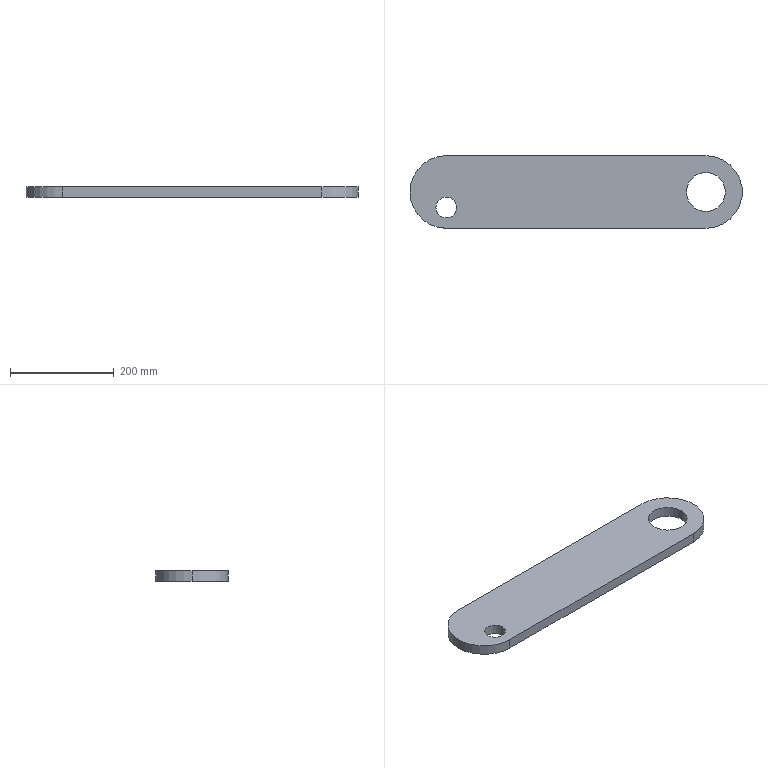Part | SolidWorks | features Extrusion 1 | 1 solid | 11 faces | box 640 x 140 x 20 mm | volume 1594386 mm3 | cylinder 7 | plane 4 | commonest cylinder face diameters 140 x3 40 x2 75 x2
STEP:
#1=CARTESIAN_POINT('',(-270.,-30.,20.));
#2=VERTEX_POINT('',#1);
#3=CARTESIAN_POINT('',(-230.,-30.,20.));
#4=VERTEX_POINT('',#3);
#5=CARTESIAN_POINT('',(-250.,-30.,20.));
#6=DIRECTION('',(0.,0.,1.));
#7=DIRECTION('',(1.,0.,0.));
#8=AXIS2_PLACEMENT_3D('',#5,#6,#7);
#9=CIRCLE('',#8,20.);
#10=EDGE_CURVE('',#2,#4,#9,.T.);
#11=ORIENTED_EDGE('',*,*,#10,.T.);
#12=CARTESIAN_POINT('',(-230.,-30.,0.));
#13=VERTEX_POINT('',#12);
#14=CARTESIAN_POINT('',(-230.,-30.,20.));
#15=DIRECTION('',(0.,0.,-1.));
#16=VECTOR('',#15,1000.);
#17=LINE('',#14,#16);
#18=EDGE_CURVE('',#4,#13,#17,.T.);
#19=ORIENTED_EDGE('',*,*,#18,.T.);
#20=CARTESIAN_POINT('',(-270.,-30.,0.));
#21=VERTEX_POINT('',#20);
#22=CARTESIAN_POINT('',(-250.,-30.,0.));
#23=DIRECTION('',(0.,0.,1.));
#24=DIRECTION('',(1.,0.,0.));
#25=AXIS2_PLACEMENT_3D('',#22,#23,#24);
#26=CIRCLE('',#25,20.);
#27=EDGE_CURVE('',#21,#13,#26,.T.);
#28=ORIENTED_EDGE('',*,*,#27,.F.);
#29=CARTESIAN_POINT('',(-270.,-30.,20.));
#30=DIRECTION('',(0.,0.,-1.));
#31=VECTOR('',#30,1000.);
#32=LINE('',#29,#31);
#33=EDGE_CURVE('',#2,#21,#32,.T.);
#34=ORIENTED_EDGE('',*,*,#33,.F.);
#35=EDGE_LOOP('',(#11,#19,#28,#34));
#36=FACE_OUTER_BOUND('',#35,.T.);
#37=CARTESIAN_POINT('',(-250.,-30.,20.));
#38=DIRECTION('',(0.,0.,-1.));
#39=DIRECTION('',(-1.,0.,0.));
#40=AXIS2_PLACEMENT_3D('',#37,#38,#39);
#41=CYLINDRICAL_SURFACE('',#40,20.);
#42=ADVANCED_FACE('',(#36),#41,.F.);
#43=CARTESIAN_POINT('',(212.5,0.,20.));
#44=VERTEX_POINT('',#43);
#45=CARTESIAN_POINT('',(287.5,0.,20.));
#46=VERTEX_POINT('',#45);
#47=CARTESIAN_POINT('',(250.,0.,20.));
#48=DIRECTION('',(0.,0.,1.));
#49=DIRECTION('',(1.,0.,0.));
#50=AXIS2_PLACEMENT_3D('',#47,#48,#49);
#51=CIRCLE('',#50,37.5);
#52=EDGE_CURVE('',#44,#46,#51,.T.);
#53=ORIENTED_EDGE('',*,*,#52,.T.);
#54=CARTESIAN_POINT('',(287.5,0.,0.));
#55=VERTEX_POINT('',#54);
#56=CARTESIAN_POINT('',(287.5,0.,20.));
#57=DIRECTION('',(0.,0.,-1.));
#58=VECTOR('',#57,1000.);
#59=LINE('',#56,#58);
#60=EDGE_CURVE('',#46,#55,#59,.T.);
#61=ORIENTED_EDGE('',*,*,#60,.T.);
#62=CARTESIAN_POINT('',(212.5,0.,0.));
#63=VERTEX_POINT('',#62);
#64=CARTESIAN_POINT('',(250.,0.,0.));
#65=DIRECTION('',(0.,0.,1.));
#66=DIRECTION('',(1.,0.,0.));
#67=AXIS2_PLACEMENT_3D('',#64,#65,#66);
#68=CIRCLE('',#67,37.5);
#69=EDGE_CURVE('',#63,#55,#68,.T.);
#70=ORIENTED_EDGE('',*,*,#69,.F.);
#71=CARTESIAN_POINT('',(212.5,0.,20.));
#72=DIRECTION('',(0.,0.,-1.));
#73=VECTOR('',#72,1000.);
#74=LINE('',#71,#73);
#75=EDGE_CURVE('',#44,#63,#74,.T.);
#76=ORIENTED_EDGE('',*,*,#75,.F.);
#77=EDGE_LOOP('',(#53,#61,#70,#76));
#78=FACE_OUTER_BOUND('',#77,.T.);
#79=CARTESIAN_POINT('',(250.,0.,20.));
#80=DIRECTION('',(0.,0.,-1.));
#81=DIRECTION('',(-1.,0.,0.));
#82=AXIS2_PLACEMENT_3D('',#79,#80,#81);
#83=CYLINDRICAL_SURFACE('',#82,37.5);
#84=ADVANCED_FACE('',(#78),#83,.F.);
#85=CARTESIAN_POINT('',(-320.,0.,20.));
#86=VERTEX_POINT('',#85);
#87=CARTESIAN_POINT('',(-250.,-70.,20.));
#88=VERTEX_POINT('',#87);
#89=CARTESIAN_POINT('',(-250.,0.,20.));
#90=DIRECTION('',(0.,0.,1.));
#91=DIRECTION('',(1.,0.,0.));
#92=AXIS2_PLACEMENT_3D('',#89,#90,#91);
#93=CIRCLE('',#92,70.);
#94=EDGE_CURVE('',#86,#88,#93,.T.);
#95=ORIENTED_EDGE('',*,*,#94,.F.);
#96=CARTESIAN_POINT('',(-320.,0.,0.));
#97=VERTEX_POINT('',#96);
#98=CARTESIAN_POINT('',(-320.,0.,20.));
#99=DIRECTION('',(0.,0.,-1.));
#100=VECTOR('',#99,1000.);
#101=LINE('',#98,#100);
#102=EDGE_CURVE('',#86,#97,#101,.T.);
#103=ORIENTED_EDGE('',*,*,#102,.T.);
#104=CARTESIAN_POINT('',(-250.,-70.,0.));
#105=VERTEX_POINT('',#104);
#106=CARTESIAN_POINT('',(-250.,0.,0.));
#107=DIRECTION('',(0.,0.,1.));
#108=DIRECTION('',(1.,0.,0.));
#109=AXIS2_PLACEMENT_3D('',#106,#107,#108);
#110=CIRCLE('',#109,70.);
#111=EDGE_CURVE('',#97,#105,#110,.T.);
#112=ORIENTED_EDGE('',*,*,#111,.T.);
#113=CARTESIAN_POINT('',(-250.,-70.,20.));
#114=DIRECTION('',(0.,0.,-1.));
#115=VECTOR('',#114,1000.);
#116=LINE('',#113,#115);
#117=EDGE_CURVE('',#88,#105,#116,.T.);
#118=ORIENTED_EDGE('',*,*,#117,.F.);
#119=EDGE_LOOP('',(#95,#103,#112,#118));
#120=FACE_OUTER_BOUND('',#119,.T.);
#121=CARTESIAN_POINT('',(-250.,0.,20.));
#122=DIRECTION('',(0.,0.,-1.));
#123=DIRECTION('',(-1.,0.,0.));
#124=AXIS2_PLACEMENT_3D('',#121,#122,#123);
#125=CYLINDRICAL_SURFACE('',#124,70.);
#126=ADVANCED_FACE('',(#120),#125,.T.);
#127=ORIENTED_EDGE('',*,*,#52,.F.);
#128=CARTESIAN_POINT('',(250.,0.,20.));
#129=DIRECTION('',(0.,0.,1.));
#130=DIRECTION('',(1.,0.,0.));
#131=AXIS2_PLACEMENT_3D('',#128,#129,#130);
#132=CIRCLE('',#131,37.5);
#133=EDGE_CURVE('',#46,#44,#132,.T.);
#134=ORIENTED_EDGE('',*,*,#133,.F.);
#135=EDGE_LOOP('',(#127,#134));
#136=FACE_BOUND('',#135,.T.);
#137=CARTESIAN_POINT('',(-250.,70.,20.));
#138=VERTEX_POINT('',#137);
#139=CARTESIAN_POINT('',(-250.,0.,20.));
#140=DIRECTION('',(0.,0.,1.));
#141=DIRECTION('',(1.,0.,0.));
#142=AXIS2_PLACEMENT_3D('',#139,#140,#141);
#143=CIRCLE('',#142,70.);
#144=EDGE_CURVE('',#138,#86,#143,.T.);
#145=ORIENTED_EDGE('',*,*,#144,.T.);
#146=ORIENTED_EDGE('',*,*,#94,.T.);
#147=CARTESIAN_POINT('',(250.,-70.,20.));
#148=VERTEX_POINT('',#147);
#149=CARTESIAN_POINT('',(-250.,-70.,20.));
#150=DIRECTION('',(1.,0.,0.));
#151=VECTOR('',#150,1000.);
#152=LINE('',#149,#151);
#153=EDGE_CURVE('',#88,#148,#152,.T.);
#154=ORIENTED_EDGE('',*,*,#153,.T.);
#155=CARTESIAN_POINT('',(250.,70.,20.));
#156=VERTEX_POINT('',#155);
#157=CARTESIAN_POINT('',(250.,0.,20.));
#158=DIRECTION('',(0.,0.,1.));
#159=DIRECTION('',(1.,0.,0.));
#160=AXIS2_PLACEMENT_3D('',#157,#158,#159);
#161=CIRCLE('',#160,70.);
#162=EDGE_CURVE('',#148,#156,#161,.T.);
#163=ORIENTED_EDGE('',*,*,#162,.T.);
#164=CARTESIAN_POINT('',(-250.,70.,20.));
#165=DIRECTION('',(-1.,0.,0.));
#166=VECTOR('',#165,1000.);
#167=LINE('',#164,#166);
#168=EDGE_CURVE('',#156,#138,#167,.T.);
#169=ORIENTED_EDGE('',*,*,#168,.T.);
#170=EDGE_LOOP('',(#145,#146,#154,#163,#169));
#171=FACE_OUTER_BOUND('',#170,.T.);
#172=ORIENTED_EDGE('',*,*,#10,.F.);
#173=CARTESIAN_POINT('',(-250.,-30.,20.));
#174=DIRECTION('',(0.,0.,1.));
#175=DIRECTION('',(1.,0.,0.));
#176=AXIS2_PLACEMENT_3D('',#173,#174,#175);
#177=CIRCLE('',#176,20.);
#178=EDGE_CURVE('',#4,#2,#177,.T.);
#179=ORIENTED_EDGE('',*,*,#178,.F.);
#180=EDGE_LOOP('',(#172,#179));
#181=FACE_BOUND('',#180,.T.);
#182=CARTESIAN_POINT('',(-250.,0.,20.));
#183=DIRECTION('',(0.,0.,1.));
#184=DIRECTION('',(1.,0.,0.));
#185=AXIS2_PLACEMENT_3D('',#182,#183,#184);
#186=PLANE('',#185);
#187=ADVANCED_FACE('',(#136,#171,#181),#186,.T.);
#188=CARTESIAN_POINT('',(-250.,70.,0.));
#189=VERTEX_POINT('',#188);
#190=CARTESIAN_POINT('',(-250.,0.,0.));
#191=DIRECTION('',(0.,0.,1.));
#192=DIRECTION('',(1.,0.,0.));
#193=AXIS2_PLACEMENT_3D('',#190,#191,#192);
#194=CIRCLE('',#193,70.);
#195=EDGE_CURVE('',#189,#97,#194,.T.);
#196=ORIENTED_EDGE('',*,*,#195,.F.);
#197=CARTESIAN_POINT('',(250.,70.,0.));
#198=VERTEX_POINT('',#197);
#199=CARTESIAN_POINT('',(-250.,70.,0.));
#200=DIRECTION('',(-1.,0.,0.));
#201=VECTOR('',#200,1000.);
#202=LINE('',#199,#201);
#203=EDGE_CURVE('',#198,#189,#202,.T.);
#204=ORIENTED_EDGE('',*,*,#203,.F.);
#205=CARTESIAN_POINT('',(250.,-70.,0.));
#206=VERTEX_POINT('',#205);
#207=CARTESIAN_POINT('',(250.,0.,0.));
#208=DIRECTION('',(0.,0.,1.));
#209=DIRECTION('',(1.,0.,0.));
#210=AXIS2_PLACEMENT_3D('',#207,#208,#209);
#211=CIRCLE('',#210,70.);
#212=EDGE_CURVE('',#206,#198,#211,.T.);
#213=ORIENTED_EDGE('',*,*,#212,.F.);
#214=CARTESIAN_POINT('',(-250.,-70.,0.));
#215=DIRECTION('',(1.,0.,0.));
#216=VECTOR('',#215,1000.);
#217=LINE('',#214,#216);
#218=EDGE_CURVE('',#105,#206,#217,.T.);
#219=ORIENTED_EDGE('',*,*,#218,.F.);
#220=ORIENTED_EDGE('',*,*,#111,.F.);
#221=EDGE_LOOP('',(#196,#204,#213,#219,#220));
#222=FACE_OUTER_BOUND('',#221,.T.);
#223=ORIENTED_EDGE('',*,*,#69,.T.);
#224=CARTESIAN_POINT('',(250.,0.,0.));
#225=DIRECTION('',(0.,0.,1.));
#226=DIRECTION('',(1.,0.,0.));
#227=AXIS2_PLACEMENT_3D('',#224,#225,#226);
#228=CIRCLE('',#227,37.5);
#229=EDGE_CURVE('',#55,#63,#228,.T.);
#230=ORIENTED_EDGE('',*,*,#229,.T.);
#231=EDGE_LOOP('',(#223,#230));
#232=FACE_BOUND('',#231,.T.);
#233=ORIENTED_EDGE('',*,*,#27,.T.);
#234=CARTESIAN_POINT('',(-250.,-30.,0.));
#235=DIRECTION('',(0.,0.,1.));
#236=DIRECTION('',(1.,0.,0.));
#237=AXIS2_PLACEMENT_3D('',#234,#235,#236);
#238=CIRCLE('',#237,20.);
#239=EDGE_CURVE('',#13,#21,#238,.T.);
#240=ORIENTED_EDGE('',*,*,#239,.T.);
#241=EDGE_LOOP('',(#233,#240));
#242=FACE_BOUND('',#241,.T.);
#243=CARTESIAN_POINT('',(-250.,0.,0.));
#244=DIRECTION('',(0.,0.,1.));
#245=DIRECTION('',(1.,0.,0.));
#246=AXIS2_PLACEMENT_3D('',#243,#244,#245);
#247=PLANE('',#246);
#248=ADVANCED_FACE('',(#222,#232,#242),#247,.F.);
#249=ORIENTED_EDGE('',*,*,#102,.F.);
#250=ORIENTED_EDGE('',*,*,#144,.F.);
#251=CARTESIAN_POINT('',(-250.,70.,20.));
#252=DIRECTION('',(0.,0.,-1.));
#253=VECTOR('',#252,1000.);
#254=LINE('',#251,#253);
#255=EDGE_CURVE('',#138,#189,#254,.T.);
#256=ORIENTED_EDGE('',*,*,#255,.T.);
#257=ORIENTED_EDGE('',*,*,#195,.T.);
#258=EDGE_LOOP('',(#249,#250,#256,#257));
#259=FACE_OUTER_BOUND('',#258,.T.);
#260=CARTESIAN_POINT('',(-250.,0.,20.));
#261=DIRECTION('',(0.,0.,-1.));
#262=DIRECTION('',(-1.,0.,0.));
#263=AXIS2_PLACEMENT_3D('',#260,#261,#262);
#264=CYLINDRICAL_SURFACE('',#263,70.);
#265=ADVANCED_FACE('',(#259),#264,.T.);
#266=ORIENTED_EDGE('',*,*,#218,.T.);
#267=CARTESIAN_POINT('',(250.,-70.,20.));
#268=DIRECTION('',(0.,0.,-1.));
#269=VECTOR('',#268,1000.);
#270=LINE('',#267,#269);
#271=EDGE_CURVE('',#148,#206,#270,.T.);
#272=ORIENTED_EDGE('',*,*,#271,.F.);
#273=ORIENTED_EDGE('',*,*,#153,.F.);
#274=ORIENTED_EDGE('',*,*,#117,.T.);
#275=EDGE_LOOP('',(#266,#272,#273,#274));
#276=FACE_OUTER_BOUND('',#275,.T.);
#277=CARTESIAN_POINT('',(-250.,-70.,20.));
#278=DIRECTION('',(0.,1.,0.));
#279=DIRECTION('',(-1.,0.,0.));
#280=AXIS2_PLACEMENT_3D('',#277,#278,#279);
#281=PLANE('',#280);
#282=ADVANCED_FACE('',(#276),#281,.F.);
#283=ORIENTED_EDGE('',*,*,#212,.T.);
#284=CARTESIAN_POINT('',(250.,70.,20.));
#285=DIRECTION('',(0.,0.,-1.));
#286=VECTOR('',#285,1000.);
#287=LINE('',#284,#286);
#288=EDGE_CURVE('',#156,#198,#287,.T.);
#289=ORIENTED_EDGE('',*,*,#288,.F.);
#290=ORIENTED_EDGE('',*,*,#162,.F.);
#291=ORIENTED_EDGE('',*,*,#271,.T.);
#292=EDGE_LOOP('',(#283,#289,#290,#291));
#293=FACE_OUTER_BOUND('',#292,.T.);
#294=CARTESIAN_POINT('',(250.,0.,20.));
#295=DIRECTION('',(0.,0.,-1.));
#296=DIRECTION('',(-1.,0.,0.));
#297=AXIS2_PLACEMENT_3D('',#294,#295,#296);
#298=CYLINDRICAL_SURFACE('',#297,70.);
#299=ADVANCED_FACE('',(#293),#298,.T.);
#300=ORIENTED_EDGE('',*,*,#203,.T.);
#301=ORIENTED_EDGE('',*,*,#255,.F.);
#302=ORIENTED_EDGE('',*,*,#168,.F.);
#303=ORIENTED_EDGE('',*,*,#288,.T.);
#304=EDGE_LOOP('',(#300,#301,#302,#303));
#305=FACE_OUTER_BOUND('',#304,.T.);
#306=CARTESIAN_POINT('',(-250.,70.,20.));
#307=DIRECTION('',(0.,-1.,0.));
#308=DIRECTION('',(1.,0.,0.));
#309=AXIS2_PLACEMENT_3D('',#306,#307,#308);
#310=PLANE('',#309);
#311=ADVANCED_FACE('',(#305),#310,.F.);
#312=ORIENTED_EDGE('',*,*,#60,.F.);
#313=ORIENTED_EDGE('',*,*,#133,.T.);
#314=ORIENTED_EDGE('',*,*,#75,.T.);
#315=ORIENTED_EDGE('',*,*,#229,.F.);
#316=EDGE_LOOP('',(#312,#313,#314,#315));
#317=FACE_OUTER_BOUND('',#316,.T.);
#318=CARTESIAN_POINT('',(250.,0.,20.));
#319=DIRECTION('',(0.,0.,-1.));
#320=DIRECTION('',(-1.,0.,0.));
#321=AXIS2_PLACEMENT_3D('',#318,#319,#320);
#322=CYLINDRICAL_SURFACE('',#321,37.5);
#323=ADVANCED_FACE('',(#317),#322,.F.);
#324=ORIENTED_EDGE('',*,*,#18,.F.);
#325=ORIENTED_EDGE('',*,*,#178,.T.);
#326=ORIENTED_EDGE('',*,*,#33,.T.);
#327=ORIENTED_EDGE('',*,*,#239,.F.);
#328=EDGE_LOOP('',(#324,#325,#326,#327));
#329=FACE_OUTER_BOUND('',#328,.T.);
#330=CARTESIAN_POINT('',(-250.,-30.,20.));
#331=DIRECTION('',(0.,0.,-1.));
#332=DIRECTION('',(-1.,0.,0.));
#333=AXIS2_PLACEMENT_3D('',#330,#331,#332);
#334=CYLINDRICAL_SURFACE('',#333,20.);
#335=ADVANCED_FACE('',(#329),#334,.F.);
#336=CLOSED_SHELL('',(#42,#84,#126,#187,#248,#265,#282,#299,#311,#323,#335));
#337=MANIFOLD_SOLID_BREP('',#336);
#338=CARTESIAN_POINT('',(0.,0.,0.));
#339=DIRECTION('',(0.,0.,1.));
#340=DIRECTION('',(1.,0.,0.));
#341=AXIS2_PLACEMENT_3D('',#338,#339,#340);
#342=(LENGTH_UNIT()NAMED_UNIT(*)SI_UNIT(.MILLI.,.METRE.));
#343=UNCERTAINTY_MEASURE_WITH_UNIT(LENGTH_MEASURE(0.00001),#342,'','');
#344=(NAMED_UNIT(*)PLANE_ANGLE_UNIT()SI_UNIT($,.RADIAN.));
#345=(NAMED_UNIT(*)SI_UNIT($,.STERADIAN.)SOLID_ANGLE_UNIT());
#346=(GEOMETRIC_REPRESENTATION_CONTEXT(3)GLOBAL_UNCERTAINTY_ASSIGNED_CONTEXT((#343))GLOBAL_UNIT_ASSIGNED_CONTEXT((#342,#344,#345))REPRESENTATION_CONTEXT('',''));
#347=ADVANCED_BREP_SHAPE_REPRESENTATION('',(#337,#341),#346);